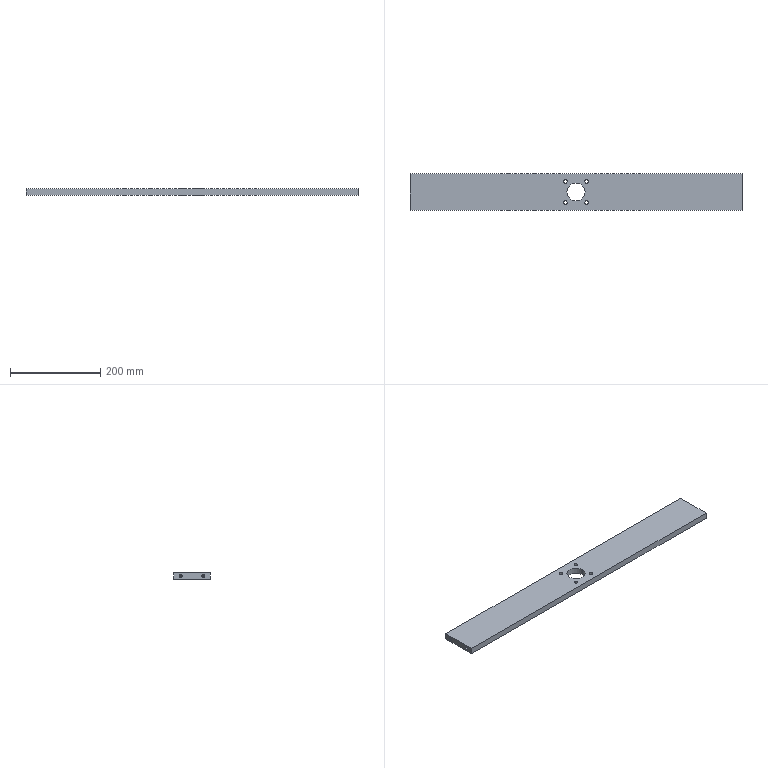Part | SolidWorks | features 3DProfileFeature 2, HoleWzd 2, Extrusion 1, ICE 1 | 1 solid | 32 faces | box 735 x 80 x 14 mm | volume 799824 mm3 | cylinder 18 | cone 8 | plane 6 | commonest cylinder face diameters 6.8 x8 8 x8 40 x2
STEP:
#1=CARTESIAN_POINT('',(715.25,15.,10.4));
#2=VERTEX_POINT('',#1);
#3=CARTESIAN_POINT('',(715.25,15.,3.6));
#4=VERTEX_POINT('',#3);
#5=CARTESIAN_POINT('',(715.25,15.,7.));
#6=DIRECTION('',(1.,0.,0.));
#7=DIRECTION('',(0.,0.,-1.));
#8=AXIS2_PLACEMENT_3D('',#5,#6,#7);
#9=CIRCLE('',#8,3.4);
#10=EDGE_CURVE('',#2,#4,#9,.T.);
#11=ORIENTED_EDGE('',*,*,#10,.F.);
#12=CARTESIAN_POINT('',(735.,15.,10.4));
#13=VERTEX_POINT('',#12);
#14=CARTESIAN_POINT('',(735.,15.,10.4));
#15=DIRECTION('',(1.,0.,0.));
#16=VECTOR('',#15,1000.);
#17=LINE('',#14,#16);
#18=EDGE_CURVE('',#2,#13,#17,.T.);
#19=ORIENTED_EDGE('',*,*,#18,.T.);
#20=CARTESIAN_POINT('',(735.,15.,3.6));
#21=VERTEX_POINT('',#20);
#22=CARTESIAN_POINT('',(735.,15.,7.));
#23=DIRECTION('',(1.,0.,0.));
#24=DIRECTION('',(0.,0.,-1.));
#25=AXIS2_PLACEMENT_3D('',#22,#23,#24);
#26=CIRCLE('',#25,3.4);
#27=EDGE_CURVE('',#13,#21,#26,.T.);
#28=ORIENTED_EDGE('',*,*,#27,.T.);
#29=CARTESIAN_POINT('',(735.,15.,3.6));
#30=DIRECTION('',(1.,0.,0.));
#31=VECTOR('',#30,1000.);
#32=LINE('',#29,#31);
#33=EDGE_CURVE('',#4,#21,#32,.T.);
#34=ORIENTED_EDGE('',*,*,#33,.F.);
#35=EDGE_LOOP('',(#11,#19,#28,#34));
#36=FACE_OUTER_BOUND('',#35,.T.);
#37=CARTESIAN_POINT('',(735.,15.,7.));
#38=DIRECTION('',(1.,0.,0.));
#39=DIRECTION('',(0.,0.,-1.));
#40=AXIS2_PLACEMENT_3D('',#37,#38,#39);
#41=CYLINDRICAL_SURFACE('',#40,3.4);
#42=ADVANCED_FACE('',(#36),#41,.F.);
#43=CARTESIAN_POINT('',(713.207,15.,7.));
#44=VERTEX_POINT('',#43);
#45=CARTESIAN_POINT('',(715.25,15.,3.6));
#46=DIRECTION('',(0.515,0.,-0.8572));
#47=VECTOR('',#46,1000.);
#48=LINE('',#45,#47);
#49=EDGE_CURVE('',#44,#4,#48,.T.);
#50=ORIENTED_EDGE('',*,*,#49,.F.);
#51=CARTESIAN_POINT('',(715.25,15.,10.4));
#52=DIRECTION('',(0.515,0.,0.8572));
#53=VECTOR('',#52,1000.);
#54=LINE('',#51,#53);
#55=EDGE_CURVE('',#44,#2,#54,.T.);
#56=ORIENTED_EDGE('',*,*,#55,.T.);
#57=ORIENTED_EDGE('',*,*,#10,.T.);
#58=EDGE_LOOP('',(#50,#56,#57));
#59=FACE_OUTER_BOUND('',#58,.T.);
#60=CARTESIAN_POINT('',(715.25,15.,7.));
#61=DIRECTION('',(1.,0.,0.));
#62=DIRECTION('',(0.,0.,-1.));
#63=AXIS2_PLACEMENT_3D('',#60,#61,#62);
#64=CONICAL_SURFACE('',#63,3.4,1.03);
#65=ADVANCED_FACE('',(#59),#64,.F.);
#66=CARTESIAN_POINT('',(715.25,65.,10.4));
#67=VERTEX_POINT('',#66);
#68=CARTESIAN_POINT('',(715.25,65.,3.6));
#69=VERTEX_POINT('',#68);
#70=CARTESIAN_POINT('',(715.25,65.,7.));
#71=DIRECTION('',(1.,0.,0.));
#72=DIRECTION('',(0.,0.,-1.));
#73=AXIS2_PLACEMENT_3D('',#70,#71,#72);
#74=CIRCLE('',#73,3.4);
#75=EDGE_CURVE('',#67,#69,#74,.T.);
#76=ORIENTED_EDGE('',*,*,#75,.F.);
#77=CARTESIAN_POINT('',(735.,65.,10.4));
#78=VERTEX_POINT('',#77);
#79=CARTESIAN_POINT('',(735.,65.,10.4));
#80=DIRECTION('',(1.,0.,0.));
#81=VECTOR('',#80,1000.);
#82=LINE('',#79,#81);
#83=EDGE_CURVE('',#67,#78,#82,.T.);
#84=ORIENTED_EDGE('',*,*,#83,.T.);
#85=CARTESIAN_POINT('',(735.,65.,3.6));
#86=VERTEX_POINT('',#85);
#87=CARTESIAN_POINT('',(735.,65.,7.));
#88=DIRECTION('',(1.,0.,0.));
#89=DIRECTION('',(0.,0.,-1.));
#90=AXIS2_PLACEMENT_3D('',#87,#88,#89);
#91=CIRCLE('',#90,3.4);
#92=EDGE_CURVE('',#78,#86,#91,.T.);
#93=ORIENTED_EDGE('',*,*,#92,.T.);
#94=CARTESIAN_POINT('',(735.,65.,3.6));
#95=DIRECTION('',(1.,0.,0.));
#96=VECTOR('',#95,1000.);
#97=LINE('',#94,#96);
#98=EDGE_CURVE('',#69,#86,#97,.T.);
#99=ORIENTED_EDGE('',*,*,#98,.F.);
#100=EDGE_LOOP('',(#76,#84,#93,#99));
#101=FACE_OUTER_BOUND('',#100,.T.);
#102=CARTESIAN_POINT('',(735.,65.,7.));
#103=DIRECTION('',(1.,0.,0.));
#104=DIRECTION('',(0.,0.,-1.));
#105=AXIS2_PLACEMENT_3D('',#102,#103,#104);
#106=CYLINDRICAL_SURFACE('',#105,3.4);
#107=ADVANCED_FACE('',(#101),#106,.F.);
#108=CARTESIAN_POINT('',(713.207,65.,7.));
#109=VERTEX_POINT('',#108);
#110=CARTESIAN_POINT('',(715.25,65.,3.6));
#111=DIRECTION('',(0.515,0.,-0.8572));
#112=VECTOR('',#111,1000.);
#113=LINE('',#110,#112);
#114=EDGE_CURVE('',#109,#69,#113,.T.);
#115=ORIENTED_EDGE('',*,*,#114,.F.);
#116=CARTESIAN_POINT('',(715.25,65.,10.4));
#117=DIRECTION('',(0.515,0.,0.8572));
#118=VECTOR('',#117,1000.);
#119=LINE('',#116,#118);
#120=EDGE_CURVE('',#109,#67,#119,.T.);
#121=ORIENTED_EDGE('',*,*,#120,.T.);
#122=ORIENTED_EDGE('',*,*,#75,.T.);
#123=EDGE_LOOP('',(#115,#121,#122));
#124=FACE_OUTER_BOUND('',#123,.T.);
#125=CARTESIAN_POINT('',(715.25,65.,7.));
#126=DIRECTION('',(1.,0.,0.));
#127=DIRECTION('',(0.,0.,-1.));
#128=AXIS2_PLACEMENT_3D('',#125,#126,#127);
#129=CONICAL_SURFACE('',#128,3.4,1.03);
#130=ADVANCED_FACE('',(#124),#129,.F.);
#131=CARTESIAN_POINT('',(19.75,65.,3.6));
#132=VERTEX_POINT('',#131);
#133=CARTESIAN_POINT('',(19.75,65.,10.4));
#134=VERTEX_POINT('',#133);
#135=CARTESIAN_POINT('',(19.75,65.,7.));
#136=DIRECTION('',(-1.,0.,0.));
#137=DIRECTION('',(0.,0.,1.));
#138=AXIS2_PLACEMENT_3D('',#135,#136,#137);
#139=CIRCLE('',#138,3.4);
#140=EDGE_CURVE('',#132,#134,#139,.T.);
#141=ORIENTED_EDGE('',*,*,#140,.F.);
#142=CARTESIAN_POINT('',(0.,65.,3.6));
#143=VERTEX_POINT('',#142);
#144=CARTESIAN_POINT('',(0.,65.,3.6));
#145=DIRECTION('',(-1.,0.,0.));
#146=VECTOR('',#145,1000.);
#147=LINE('',#144,#146);
#148=EDGE_CURVE('',#132,#143,#147,.T.);
#149=ORIENTED_EDGE('',*,*,#148,.T.);
#150=CARTESIAN_POINT('',(0.,65.,10.4));
#151=VERTEX_POINT('',#150);
#152=CARTESIAN_POINT('',(0.,65.,7.));
#153=DIRECTION('',(-1.,0.,0.));
#154=DIRECTION('',(0.,0.,1.));
#155=AXIS2_PLACEMENT_3D('',#152,#153,#154);
#156=CIRCLE('',#155,3.4);
#157=EDGE_CURVE('',#143,#151,#156,.T.);
#158=ORIENTED_EDGE('',*,*,#157,.T.);
#159=CARTESIAN_POINT('',(0.,65.,10.4));
#160=DIRECTION('',(-1.,0.,0.));
#161=VECTOR('',#160,1000.);
#162=LINE('',#159,#161);
#163=EDGE_CURVE('',#134,#151,#162,.T.);
#164=ORIENTED_EDGE('',*,*,#163,.F.);
#165=EDGE_LOOP('',(#141,#149,#158,#164));
#166=FACE_OUTER_BOUND('',#165,.T.);
#167=CARTESIAN_POINT('',(0.,65.,7.));
#168=DIRECTION('',(-1.,0.,0.));
#169=DIRECTION('',(0.,0.,1.));
#170=AXIS2_PLACEMENT_3D('',#167,#168,#169);
#171=CYLINDRICAL_SURFACE('',#170,3.4);
#172=ADVANCED_FACE('',(#166),#171,.F.);
#173=CARTESIAN_POINT('',(21.793,65.,7.));
#174=VERTEX_POINT('',#173);
#175=CARTESIAN_POINT('',(19.75,65.,10.4));
#176=DIRECTION('',(-0.515,0.,0.8572));
#177=VECTOR('',#176,1000.);
#178=LINE('',#175,#177);
#179=EDGE_CURVE('',#174,#134,#178,.T.);
#180=ORIENTED_EDGE('',*,*,#179,.F.);
#181=CARTESIAN_POINT('',(19.75,65.,3.6));
#182=DIRECTION('',(-0.515,0.,-0.8572));
#183=VECTOR('',#182,1000.);
#184=LINE('',#181,#183);
#185=EDGE_CURVE('',#174,#132,#184,.T.);
#186=ORIENTED_EDGE('',*,*,#185,.T.);
#187=ORIENTED_EDGE('',*,*,#140,.T.);
#188=EDGE_LOOP('',(#180,#186,#187));
#189=FACE_OUTER_BOUND('',#188,.T.);
#190=CARTESIAN_POINT('',(19.75,65.,7.));
#191=DIRECTION('',(-1.,0.,0.));
#192=DIRECTION('',(0.,0.,1.));
#193=AXIS2_PLACEMENT_3D('',#190,#191,#192);
#194=CONICAL_SURFACE('',#193,3.4,1.03);
#195=ADVANCED_FACE('',(#189),#194,.F.);
#196=CARTESIAN_POINT('',(19.75,15.,3.6));
#197=VERTEX_POINT('',#196);
#198=CARTESIAN_POINT('',(19.75,15.,10.4));
#199=VERTEX_POINT('',#198);
#200=CARTESIAN_POINT('',(19.75,15.,7.));
#201=DIRECTION('',(-1.,0.,0.));
#202=DIRECTION('',(0.,0.,1.));
#203=AXIS2_PLACEMENT_3D('',#200,#201,#202);
#204=CIRCLE('',#203,3.4);
#205=EDGE_CURVE('',#197,#199,#204,.T.);
#206=ORIENTED_EDGE('',*,*,#205,.F.);
#207=CARTESIAN_POINT('',(0.,15.,3.6));
#208=VERTEX_POINT('',#207);
#209=CARTESIAN_POINT('',(0.,15.,3.6));
#210=DIRECTION('',(-1.,0.,0.));
#211=VECTOR('',#210,1000.);
#212=LINE('',#209,#211);
#213=EDGE_CURVE('',#197,#208,#212,.T.);
#214=ORIENTED_EDGE('',*,*,#213,.T.);
#215=CARTESIAN_POINT('',(0.,15.,10.4));
#216=VERTEX_POINT('',#215);
#217=CARTESIAN_POINT('',(0.,15.,7.));
#218=DIRECTION('',(-1.,0.,0.));
#219=DIRECTION('',(0.,0.,1.));
#220=AXIS2_PLACEMENT_3D('',#217,#218,#219);
#221=CIRCLE('',#220,3.4);
#222=EDGE_CURVE('',#208,#216,#221,.T.);
#223=ORIENTED_EDGE('',*,*,#222,.T.);
#224=CARTESIAN_POINT('',(0.,15.,10.4));
#225=DIRECTION('',(-1.,0.,0.));
#226=VECTOR('',#225,1000.);
#227=LINE('',#224,#226);
#228=EDGE_CURVE('',#199,#216,#227,.T.);
#229=ORIENTED_EDGE('',*,*,#228,.F.);
#230=EDGE_LOOP('',(#206,#214,#223,#229));
#231=FACE_OUTER_BOUND('',#230,.T.);
#232=CARTESIAN_POINT('',(0.,15.,7.));
#233=DIRECTION('',(-1.,0.,0.));
#234=DIRECTION('',(0.,0.,1.));
#235=AXIS2_PLACEMENT_3D('',#232,#233,#234);
#236=CYLINDRICAL_SURFACE('',#235,3.4);
#237=ADVANCED_FACE('',(#231),#236,.F.);
#238=CARTESIAN_POINT('',(21.793,15.,7.));
#239=VERTEX_POINT('',#238);
#240=CARTESIAN_POINT('',(19.75,15.,10.4));
#241=DIRECTION('',(-0.515,0.,0.8572));
#242=VECTOR('',#241,1000.);
#243=LINE('',#240,#242);
#244=EDGE_CURVE('',#239,#199,#243,.T.);
#245=ORIENTED_EDGE('',*,*,#244,.F.);
#246=CARTESIAN_POINT('',(19.75,15.,3.6));
#247=DIRECTION('',(-0.515,0.,-0.8572));
#248=VECTOR('',#247,1000.);
#249=LINE('',#246,#248);
#250=EDGE_CURVE('',#239,#197,#249,.T.);
#251=ORIENTED_EDGE('',*,*,#250,.T.);
#252=ORIENTED_EDGE('',*,*,#205,.T.);
#253=EDGE_LOOP('',(#245,#251,#252));
#254=FACE_OUTER_BOUND('',#253,.T.);
#255=CARTESIAN_POINT('',(19.75,15.,7.));
#256=DIRECTION('',(-1.,0.,0.));
#257=DIRECTION('',(0.,0.,1.));
#258=AXIS2_PLACEMENT_3D('',#255,#256,#257);
#259=CONICAL_SURFACE('',#258,3.4,1.03);
#260=ADVANCED_FACE('',(#254),#259,.F.);
#261=CARTESIAN_POINT('',(340.,16.5,0.));
#262=VERTEX_POINT('',#261);
#263=CARTESIAN_POINT('',(348.,16.5,0.));
#264=VERTEX_POINT('',#263);
#265=CARTESIAN_POINT('',(344.,16.5,0.));
#266=DIRECTION('',(0.,0.,1.));
#267=DIRECTION('',(1.,0.,0.));
#268=AXIS2_PLACEMENT_3D('',#265,#266,#267);
#269=CIRCLE('',#268,4.);
#270=EDGE_CURVE('',#262,#264,#269,.T.);
#271=ORIENTED_EDGE('',*,*,#270,.F.);
#272=CARTESIAN_POINT('',(340.,16.5,14.));
#273=VERTEX_POINT('',#272);
#274=CARTESIAN_POINT('',(340.,16.5,0.));
#275=DIRECTION('',(0.,0.,1.));
#276=VECTOR('',#275,1000.);
#277=LINE('',#274,#276);
#278=EDGE_CURVE('',#262,#273,#277,.T.);
#279=ORIENTED_EDGE('',*,*,#278,.T.);
#280=CARTESIAN_POINT('',(348.,16.5,14.));
#281=VERTEX_POINT('',#280);
#282=CARTESIAN_POINT('',(344.,16.5,14.));
#283=DIRECTION('',(0.,0.,1.));
#284=DIRECTION('',(1.,0.,0.));
#285=AXIS2_PLACEMENT_3D('',#282,#283,#284);
#286=CIRCLE('',#285,4.);
#287=EDGE_CURVE('',#273,#281,#286,.T.);
#288=ORIENTED_EDGE('',*,*,#287,.T.);
#289=CARTESIAN_POINT('',(348.,16.5,0.));
#290=DIRECTION('',(0.,0.,1.));
#291=VECTOR('',#290,1000.);
#292=LINE('',#289,#291);
#293=EDGE_CURVE('',#264,#281,#292,.T.);
#294=ORIENTED_EDGE('',*,*,#293,.F.);
#295=EDGE_LOOP('',(#271,#279,#288,#294));
#296=FACE_OUTER_BOUND('',#295,.T.);
#297=CARTESIAN_POINT('',(344.,16.5,0.));
#298=DIRECTION('',(0.,0.,1.));
#299=DIRECTION('',(1.,0.,0.));
#300=AXIS2_PLACEMENT_3D('',#297,#298,#299);
#301=CYLINDRICAL_SURFACE('',#300,4.);
#302=ADVANCED_FACE('',(#296),#301,.F.);
#303=CARTESIAN_POINT('',(387.,16.5,0.));
#304=VERTEX_POINT('',#303);
#305=CARTESIAN_POINT('',(395.,16.5,0.));
#306=VERTEX_POINT('',#305);
#307=CARTESIAN_POINT('',(391.,16.5,0.));
#308=DIRECTION('',(0.,0.,1.));
#309=DIRECTION('',(1.,0.,0.));
#310=AXIS2_PLACEMENT_3D('',#307,#308,#309);
#311=CIRCLE('',#310,4.);
#312=EDGE_CURVE('',#304,#306,#311,.T.);
#313=ORIENTED_EDGE('',*,*,#312,.F.);
#314=CARTESIAN_POINT('',(387.,16.5,14.));
#315=VERTEX_POINT('',#314);
#316=CARTESIAN_POINT('',(387.,16.5,0.));
#317=DIRECTION('',(0.,0.,1.));
#318=VECTOR('',#317,1000.);
#319=LINE('',#316,#318);
#320=EDGE_CURVE('',#304,#315,#319,.T.);
#321=ORIENTED_EDGE('',*,*,#320,.T.);
#322=CARTESIAN_POINT('',(395.,16.5,14.));
#323=VERTEX_POINT('',#322);
#324=CARTESIAN_POINT('',(391.,16.5,14.));
#325=DIRECTION('',(0.,0.,1.));
#326=DIRECTION('',(1.,0.,0.));
#327=AXIS2_PLACEMENT_3D('',#324,#325,#326);
#328=CIRCLE('',#327,4.);
#329=EDGE_CURVE('',#315,#323,#328,.T.);
#330=ORIENTED_EDGE('',*,*,#329,.T.);
#331=CARTESIAN_POINT('',(395.,16.5,0.));
#332=DIRECTION('',(0.,0.,1.));
#333=VECTOR('',#332,1000.);
#334=LINE('',#331,#333);
#335=EDGE_CURVE('',#306,#323,#334,.T.);
#336=ORIENTED_EDGE('',*,*,#335,.F.);
#337=EDGE_LOOP('',(#313,#321,#330,#336));
#338=FACE_OUTER_BOUND('',#337,.T.);
#339=CARTESIAN_POINT('',(391.,16.5,0.));
#340=DIRECTION('',(0.,0.,1.));
#341=DIRECTION('',(1.,0.,0.));
#342=AXIS2_PLACEMENT_3D('',#339,#340,#341);
#343=CYLINDRICAL_SURFACE('',#342,4.);
#344=ADVANCED_FACE('',(#338),#343,.F.);
#345=CARTESIAN_POINT('',(347.5,40.,0.));
#346=VERTEX_POINT('',#345);
#347=CARTESIAN_POINT('',(387.5,40.,0.));
#348=VERTEX_POINT('',#347);
#349=CARTESIAN_POINT('',(367.5,40.,0.));
#350=DIRECTION('',(0.,0.,1.));
#351=DIRECTION('',(1.,0.,0.));
#352=AXIS2_PLACEMENT_3D('',#349,#350,#351);
#353=CIRCLE('',#352,20.);
#354=EDGE_CURVE('',#346,#348,#353,.T.);
#355=ORIENTED_EDGE('',*,*,#354,.F.);
#356=CARTESIAN_POINT('',(347.5,40.,14.));
#357=VERTEX_POINT('',#356);
#358=CARTESIAN_POINT('',(347.5,40.,0.));
#359=DIRECTION('',(0.,0.,1.));
#360=VECTOR('',#359,1000.);
#361=LINE('',#358,#360);
#362=EDGE_CURVE('',#346,#357,#361,.T.);
#363=ORIENTED_EDGE('',*,*,#362,.T.);
#364=CARTESIAN_POINT('',(387.5,40.,14.));
#365=VERTEX_POINT('',#364);
#366=CARTESIAN_POINT('',(367.5,40.,14.));
#367=DIRECTION('',(0.,0.,1.));
#368=DIRECTION('',(1.,0.,0.));
#369=AXIS2_PLACEMENT_3D('',#366,#367,#368);
#370=CIRCLE('',#369,20.);
#371=EDGE_CURVE('',#357,#365,#370,.T.);
#372=ORIENTED_EDGE('',*,*,#371,.T.);
#373=CARTESIAN_POINT('',(387.5,40.,0.));
#374=DIRECTION('',(0.,0.,1.));
#375=VECTOR('',#374,1000.);
#376=LINE('',#373,#375);
#377=EDGE_CURVE('',#348,#365,#376,.T.);
#378=ORIENTED_EDGE('',*,*,#377,.F.);
#379=EDGE_LOOP('',(#355,#363,#372,#378));
#380=FACE_OUTER_BOUND('',#379,.T.);
#381=CARTESIAN_POINT('',(367.5,40.,0.));
#382=DIRECTION('',(0.,0.,1.));
#383=DIRECTION('',(1.,0.,0.));
#384=AXIS2_PLACEMENT_3D('',#381,#382,#383);
#385=CYLINDRICAL_SURFACE('',#384,20.);
#386=ADVANCED_FACE('',(#380),#385,.F.);
#387=CARTESIAN_POINT('',(387.,63.5,0.));
#388=VERTEX_POINT('',#387);
#389=CARTESIAN_POINT('',(395.,63.5,0.));
#390=VERTEX_POINT('',#389);
#391=CARTESIAN_POINT('',(391.,63.5,0.));
#392=DIRECTION('',(0.,0.,1.));
#393=DIRECTION('',(1.,0.,0.));
#394=AXIS2_PLACEMENT_3D('',#391,#392,#393);
#395=CIRCLE('',#394,4.);
#396=EDGE_CURVE('',#388,#390,#395,.T.);
#397=ORIENTED_EDGE('',*,*,#396,.F.);
#398=CARTESIAN_POINT('',(387.,63.5,14.));
#399=VERTEX_POINT('',#398);
#400=CARTESIAN_POINT('',(387.,63.5,0.));
#401=DIRECTION('',(0.,0.,1.));
#402=VECTOR('',#401,1000.);
#403=LINE('',#400,#402);
#404=EDGE_CURVE('',#388,#399,#403,.T.);
#405=ORIENTED_EDGE('',*,*,#404,.T.);
#406=CARTESIAN_POINT('',(395.,63.5,14.));
#407=VERTEX_POINT('',#406);
#408=CARTESIAN_POINT('',(391.,63.5,14.));
#409=DIRECTION('',(0.,0.,1.));
#410=DIRECTION('',(1.,0.,0.));
#411=AXIS2_PLACEMENT_3D('',#408,#409,#410);
#412=CIRCLE('',#411,4.);
#413=EDGE_CURVE('',#399,#407,#412,.T.);
#414=ORIENTED_EDGE('',*,*,#413,.T.);
#415=CARTESIAN_POINT('',(395.,63.5,0.));
#416=DIRECTION('',(0.,0.,1.));
#417=VECTOR('',#416,1000.);
#418=LINE('',#415,#417);
#419=EDGE_CURVE('',#390,#407,#418,.T.);
#420=ORIENTED_EDGE('',*,*,#419,.F.);
#421=EDGE_LOOP('',(#397,#405,#414,#420));
#422=FACE_OUTER_BOUND('',#421,.T.);
#423=CARTESIAN_POINT('',(391.,63.5,0.));
#424=DIRECTION('',(0.,0.,1.));
#425=DIRECTION('',(1.,0.,0.));
#426=AXIS2_PLACEMENT_3D('',#423,#424,#425);
#427=CYLINDRICAL_SURFACE('',#426,4.);
#428=ADVANCED_FACE('',(#422),#427,.F.);
#429=CARTESIAN_POINT('',(340.,63.5,0.));
#430=VERTEX_POINT('',#429);
#431=CARTESIAN_POINT('',(348.,63.5,0.));
#432=VERTEX_POINT('',#431);
#433=CARTESIAN_POINT('',(344.,63.5,0.));
#434=DIRECTION('',(0.,0.,1.));
#435=DIRECTION('',(1.,0.,0.));
#436=AXIS2_PLACEMENT_3D('',#433,#434,#435);
#437=CIRCLE('',#436,4.);
#438=EDGE_CURVE('',#430,#432,#437,.T.);
#439=ORIENTED_EDGE('',*,*,#438,.F.);
#440=CARTESIAN_POINT('',(340.,63.5,14.));
#441=VERTEX_POINT('',#440);
#442=CARTESIAN_POINT('',(340.,63.5,0.));
#443=DIRECTION('',(0.,0.,1.));
#444=VECTOR('',#443,1000.);
#445=LINE('',#442,#444);
#446=EDGE_CURVE('',#430,#441,#445,.T.);
#447=ORIENTED_EDGE('',*,*,#446,.T.);
#448=CARTESIAN_POINT('',(348.,63.5,14.));
#449=VERTEX_POINT('',#448);
#450=CARTESIAN_POINT('',(344.,63.5,14.));
#451=DIRECTION('',(0.,0.,1.));
#452=DIRECTION('',(1.,0.,0.));
#453=AXIS2_PLACEMENT_3D('',#450,#451,#452);
#454=CIRCLE('',#453,4.);
#455=EDGE_CURVE('',#441,#449,#454,.T.);
#456=ORIENTED_EDGE('',*,*,#455,.T.);
#457=CARTESIAN_POINT('',(348.,63.5,0.));
#458=DIRECTION('',(0.,0.,1.));
#459=VECTOR('',#458,1000.);
#460=LINE('',#457,#459);
#461=EDGE_CURVE('',#432,#449,#460,.T.);
#462=ORIENTED_EDGE('',*,*,#461,.F.);
#463=EDGE_LOOP('',(#439,#447,#456,#462));
#464=FACE_OUTER_BOUND('',#463,.T.);
#465=CARTESIAN_POINT('',(344.,63.5,0.));
#466=DIRECTION('',(0.,0.,1.));
#467=DIRECTION('',(1.,0.,0.));
#468=AXIS2_PLACEMENT_3D('',#465,#466,#467);
#469=CYLINDRICAL_SURFACE('',#468,4.);
#470=ADVANCED_FACE('',(#464),#469,.F.);
#471=CARTESIAN_POINT('',(0.,65.,7.));
#472=DIRECTION('',(-1.,0.,0.));
#473=DIRECTION('',(0.,0.,1.));
#474=AXIS2_PLACEMENT_3D('',#471,#472,#473);
#475=CIRCLE('',#474,3.4);
#476=EDGE_CURVE('',#151,#143,#475,.T.);
#477=ORIENTED_EDGE('',*,*,#476,.F.);
#478=ORIENTED_EDGE('',*,*,#157,.F.);
#479=EDGE_LOOP('',(#477,#478));
#480=FACE_BOUND('',#479,.T.);
#481=CARTESIAN_POINT('',(0.,15.,7.));
#482=DIRECTION('',(-1.,0.,0.));
#483=DIRECTION('',(0.,0.,1.));
#484=AXIS2_PLACEMENT_3D('',#481,#482,#483);
#485=CIRCLE('',#484,3.4);
#486=EDGE_CURVE('',#216,#208,#485,.T.);
#487=ORIENTED_EDGE('',*,*,#486,.F.);
#488=ORIENTED_EDGE('',*,*,#222,.F.);
#489=EDGE_LOOP('',(#487,#488));
#490=FACE_BOUND('',#489,.T.);
#491=CARTESIAN_POINT('',(0.,80.,0.));
#492=VERTEX_POINT('',#491);
#493=CARTESIAN_POINT('',(0.,0.,0.));
#494=VERTEX_POINT('',#493);
#495=CARTESIAN_POINT('',(0.,0.,0.));
#496=DIRECTION('',(0.,-1.,0.));
#497=VECTOR('',#496,1000.);
#498=LINE('',#495,#497);
#499=EDGE_CURVE('',#492,#494,#498,.T.);
#500=ORIENTED_EDGE('',*,*,#499,.T.);
#501=CARTESIAN_POINT('',(0.,0.,14.));
#502=VERTEX_POINT('',#501);
#503=CARTESIAN_POINT('',(0.,0.,14.));
#504=DIRECTION('',(0.,0.,-1.));
#505=VECTOR('',#504,1000.);
#506=LINE('',#503,#505);
#507=EDGE_CURVE('',#502,#494,#506,.T.);
#508=ORIENTED_EDGE('',*,*,#507,.F.);
#509=CARTESIAN_POINT('',(0.,80.,14.));
#510=VERTEX_POINT('',#509);
#511=CARTESIAN_POINT('',(0.,0.,14.));
#512=DIRECTION('',(0.,-1.,0.));
#513=VECTOR('',#512,1000.);
#514=LINE('',#511,#513);
#515=EDGE_CURVE('',#510,#502,#514,.T.);
#516=ORIENTED_EDGE('',*,*,#515,.F.);
#517=CARTESIAN_POINT('',(0.,80.,14.));
#518=DIRECTION('',(0.,0.,-1.));
#519=VECTOR('',#518,1000.);
#520=LINE('',#517,#519);
#521=EDGE_CURVE('',#510,#492,#520,.T.);
#522=ORIENTED_EDGE('',*,*,#521,.T.);
#523=EDGE_LOOP('',(#500,#508,#516,#522));
#524=FACE_OUTER_BOUND('',#523,.T.);
#525=CARTESIAN_POINT('',(0.,0.,14.));
#526=DIRECTION('',(1.,0.,0.));
#527=DIRECTION('',(0.,0.,-1.));
#528=AXIS2_PLACEMENT_3D('',#525,#526,#527);
#529=PLANE('',#528);
#530=ADVANCED_FACE('',(#480,#490,#524),#529,.F.);
#531=CARTESIAN_POINT('',(735.,0.,0.));
#532=VERTEX_POINT('',#531);
#533=CARTESIAN_POINT('',(0.,0.,0.));
#534=DIRECTION('',(1.,0.,0.));
#535=VECTOR('',#534,1000.);
#536=LINE('',#533,#535);
#537=EDGE_CURVE('',#494,#532,#536,.T.);
#538=ORIENTED_EDGE('',*,*,#537,.T.);
#539=CARTESIAN_POINT('',(735.,0.,14.));
#540=VERTEX_POINT('',#539);
#541=CARTESIAN_POINT('',(735.,0.,14.));
#542=DIRECTION('',(0.,0.,-1.));
#543=VECTOR('',#542,1000.);
#544=LINE('',#541,#543);
#545=EDGE_CURVE('',#540,#532,#544,.T.);
#546=ORIENTED_EDGE('',*,*,#545,.F.);
#547=CARTESIAN_POINT('',(0.,0.,14.));
#548=DIRECTION('',(1.,0.,0.));
#549=VECTOR('',#548,1000.);
#550=LINE('',#547,#549);
#551=EDGE_CURVE('',#502,#540,#550,.T.);
#552=ORIENTED_EDGE('',*,*,#551,.F.);
#553=ORIENTED_EDGE('',*,*,#507,.T.);
#554=EDGE_LOOP('',(#538,#546,#552,#553));
#555=FACE_OUTER_BOUND('',#554,.T.);
#556=CARTESIAN_POINT('',(0.,0.,14.));
#557=DIRECTION('',(0.,1.,0.));
#558=DIRECTION('',(0.,0.,1.));
#559=AXIS2_PLACEMENT_3D('',#556,#557,#558);
#560=PLANE('',#559);
#561=ADVANCED_FACE('',(#555),#560,.F.);
#562=CARTESIAN_POINT('',(735.,15.,7.));
#563=DIRECTION('',(1.,0.,0.));
#564=DIRECTION('',(0.,0.,-1.));
#565=AXIS2_PLACEMENT_3D('',#562,#563,#564);
#566=CIRCLE('',#565,3.4);
#567=EDGE_CURVE('',#21,#13,#566,.T.);
#568=ORIENTED_EDGE('',*,*,#567,.F.);
#569=ORIENTED_EDGE('',*,*,#27,.F.);
#570=EDGE_LOOP('',(#568,#569));
#571=FACE_BOUND('',#570,.T.);
#572=CARTESIAN_POINT('',(735.,65.,7.));
#573=DIRECTION('',(1.,0.,0.));
#574=DIRECTION('',(0.,0.,-1.));
#575=AXIS2_PLACEMENT_3D('',#572,#573,#574);
#576=CIRCLE('',#575,3.4);
#577=EDGE_CURVE('',#86,#78,#576,.T.);
#578=ORIENTED_EDGE('',*,*,#577,.F.);
#579=ORIENTED_EDGE('',*,*,#92,.F.);
#580=EDGE_LOOP('',(#578,#579));
#581=FACE_BOUND('',#580,.T.);
#582=CARTESIAN_POINT('',(735.,80.,0.));
#583=VERTEX_POINT('',#582);
#584=CARTESIAN_POINT('',(735.,0.,0.));
#585=DIRECTION('',(0.,1.,0.));
#586=VECTOR('',#585,1000.);
#587=LINE('',#584,#586);
#588=EDGE_CURVE('',#532,#583,#587,.T.);
#589=ORIENTED_EDGE('',*,*,#588,.T.);
#590=CARTESIAN_POINT('',(735.,80.,14.));
#591=VERTEX_POINT('',#590);
#592=CARTESIAN_POINT('',(735.,80.,14.));
#593=DIRECTION('',(0.,0.,-1.));
#594=VECTOR('',#593,1000.);
#595=LINE('',#592,#594);
#596=EDGE_CURVE('',#591,#583,#595,.T.);
#597=ORIENTED_EDGE('',*,*,#596,.F.);
#598=CARTESIAN_POINT('',(735.,0.,14.));
#599=DIRECTION('',(0.,1.,0.));
#600=VECTOR('',#599,1000.);
#601=LINE('',#598,#600);
#602=EDGE_CURVE('',#540,#591,#601,.T.);
#603=ORIENTED_EDGE('',*,*,#602,.F.);
#604=ORIENTED_EDGE('',*,*,#545,.T.);
#605=EDGE_LOOP('',(#589,#597,#603,#604));
#606=FACE_OUTER_BOUND('',#605,.T.);
#607=CARTESIAN_POINT('',(735.,0.,14.));
#608=DIRECTION('',(-1.,0.,0.));
#609=DIRECTION('',(0.,0.,1.));
#610=AXIS2_PLACEMENT_3D('',#607,#608,#609);
#611=PLANE('',#610);
#612=ADVANCED_FACE('',(#571,#581,#606),#611,.F.);
#613=CARTESIAN_POINT('',(0.,80.,0.));
#614=DIRECTION('',(-1.,0.,0.));
#615=VECTOR('',#614,1000.);
#616=LINE('',#613,#615);
#617=EDGE_CURVE('',#583,#492,#616,.T.);
#618=ORIENTED_EDGE('',*,*,#617,.T.);
#619=ORIENTED_EDGE('',*,*,#521,.F.);
#620=CARTESIAN_POINT('',(0.,80.,14.));
#621=DIRECTION('',(-1.,0.,0.));
#622=VECTOR('',#621,1000.);
#623=LINE('',#620,#622);
#624=EDGE_CURVE('',#591,#510,#623,.T.);
#625=ORIENTED_EDGE('',*,*,#624,.F.);
#626=ORIENTED_EDGE('',*,*,#596,.T.);
#627=EDGE_LOOP('',(#618,#619,#625,#626));
#628=FACE_OUTER_BOUND('',#627,.T.);
#629=CARTESIAN_POINT('',(0.,80.,14.));
#630=DIRECTION('',(0.,-1.,0.));
#631=DIRECTION('',(0.,0.,-1.));
#632=AXIS2_PLACEMENT_3D('',#629,#630,#631);
#633=PLANE('',#632);
#634=ADVANCED_FACE('',(#628),#633,.F.);
#635=CARTESIAN_POINT('',(344.,16.5,14.));
#636=DIRECTION('',(0.,0.,1.));
#637=DIRECTION('',(1.,0.,0.));
#638=AXIS2_PLACEMENT_3D('',#635,#636,#637);
#639=CIRCLE('',#638,4.);
#640=EDGE_CURVE('',#281,#273,#639,.T.);
#641=ORIENTED_EDGE('',*,*,#640,.F.);
#642=ORIENTED_EDGE('',*,*,#287,.F.);
#643=EDGE_LOOP('',(#641,#642));
#644=FACE_BOUND('',#643,.T.);
#645=CARTESIAN_POINT('',(391.,16.5,14.));
#646=DIRECTION('',(0.,0.,1.));
#647=DIRECTION('',(1.,0.,0.));
#648=AXIS2_PLACEMENT_3D('',#645,#646,#647);
#649=CIRCLE('',#648,4.);
#650=EDGE_CURVE('',#323,#315,#649,.T.);
#651=ORIENTED_EDGE('',*,*,#650,.F.);
#652=ORIENTED_EDGE('',*,*,#329,.F.);
#653=EDGE_LOOP('',(#651,#652));
#654=FACE_BOUND('',#653,.T.);
#655=CARTESIAN_POINT('',(367.5,40.,14.));
#656=DIRECTION('',(0.,0.,1.));
#657=DIRECTION('',(1.,0.,0.));
#658=AXIS2_PLACEMENT_3D('',#655,#656,#657);
#659=CIRCLE('',#658,20.);
#660=EDGE_CURVE('',#365,#357,#659,.T.);
#661=ORIENTED_EDGE('',*,*,#660,.F.);
#662=ORIENTED_EDGE('',*,*,#371,.F.);
#663=EDGE_LOOP('',(#661,#662));
#664=FACE_BOUND('',#663,.T.);
#665=CARTESIAN_POINT('',(391.,63.5,14.));
#666=DIRECTION('',(0.,0.,1.));
#667=DIRECTION('',(1.,0.,0.));
#668=AXIS2_PLACEMENT_3D('',#665,#666,#667);
#669=CIRCLE('',#668,4.);
#670=EDGE_CURVE('',#407,#399,#669,.T.);
#671=ORIENTED_EDGE('',*,*,#670,.F.);
#672=ORIENTED_EDGE('',*,*,#413,.F.);
#673=EDGE_LOOP('',(#671,#672));
#674=FACE_BOUND('',#673,.T.);
#675=CARTESIAN_POINT('',(344.,63.5,14.));
#676=DIRECTION('',(0.,0.,1.));
#677=DIRECTION('',(1.,0.,0.));
#678=AXIS2_PLACEMENT_3D('',#675,#676,#677);
#679=CIRCLE('',#678,4.);
#680=EDGE_CURVE('',#449,#441,#679,.T.);
#681=ORIENTED_EDGE('',*,*,#680,.F.);
#682=ORIENTED_EDGE('',*,*,#455,.F.);
#683=EDGE_LOOP('',(#681,#682));
#684=FACE_BOUND('',#683,.T.);
#685=ORIENTED_EDGE('',*,*,#515,.T.);
#686=ORIENTED_EDGE('',*,*,#551,.T.);
#687=ORIENTED_EDGE('',*,*,#602,.T.);
#688=ORIENTED_EDGE('',*,*,#624,.T.);
#689=EDGE_LOOP('',(#685,#686,#687,#688));
#690=FACE_OUTER_BOUND('',#689,.T.);
#691=CARTESIAN_POINT('',(0.,0.,14.));
#692=DIRECTION('',(0.,0.,-1.));
#693=DIRECTION('',(-1.,0.,0.));
#694=AXIS2_PLACEMENT_3D('',#691,#692,#693);
#695=PLANE('',#694);
#696=ADVANCED_FACE('',(#644,#654,#664,#674,#684,#690),#695,.F.);
#697=CARTESIAN_POINT('',(344.,16.5,0.));
#698=DIRECTION('',(0.,0.,1.));
#699=DIRECTION('',(1.,0.,0.));
#700=AXIS2_PLACEMENT_3D('',#697,#698,#699);
#701=CIRCLE('',#700,4.);
#702=EDGE_CURVE('',#264,#262,#701,.T.);
#703=ORIENTED_EDGE('',*,*,#702,.T.);
#704=ORIENTED_EDGE('',*,*,#270,.T.);
#705=EDGE_LOOP('',(#703,#704));
#706=FACE_BOUND('',#705,.T.);
#707=CARTESIAN_POINT('',(391.,16.5,0.));
#708=DIRECTION('',(0.,0.,1.));
#709=DIRECTION('',(1.,0.,0.));
#710=AXIS2_PLACEMENT_3D('',#707,#708,#709);
#711=CIRCLE('',#710,4.);
#712=EDGE_CURVE('',#306,#304,#711,.T.);
#713=ORIENTED_EDGE('',*,*,#712,.T.);
#714=ORIENTED_EDGE('',*,*,#312,.T.);
#715=EDGE_LOOP('',(#713,#714));
#716=FACE_BOUND('',#715,.T.);
#717=CARTESIAN_POINT('',(367.5,40.,0.));
#718=DIRECTION('',(0.,0.,1.));
#719=DIRECTION('',(1.,0.,0.));
#720=AXIS2_PLACEMENT_3D('',#717,#718,#719);
#721=CIRCLE('',#720,20.);
#722=EDGE_CURVE('',#348,#346,#721,.T.);
#723=ORIENTED_EDGE('',*,*,#722,.T.);
#724=ORIENTED_EDGE('',*,*,#354,.T.);
#725=EDGE_LOOP('',(#723,#724));
#726=FACE_BOUND('',#725,.T.);
#727=CARTESIAN_POINT('',(391.,63.5,0.));
#728=DIRECTION('',(0.,0.,1.));
#729=DIRECTION('',(1.,0.,0.));
#730=AXIS2_PLACEMENT_3D('',#727,#728,#729);
#731=CIRCLE('',#730,4.);
#732=EDGE_CURVE('',#390,#388,#731,.T.);
#733=ORIENTED_EDGE('',*,*,#732,.T.);
#734=ORIENTED_EDGE('',*,*,#396,.T.);
#735=EDGE_LOOP('',(#733,#734));
#736=FACE_BOUND('',#735,.T.);
#737=CARTESIAN_POINT('',(344.,63.5,0.));
#738=DIRECTION('',(0.,0.,1.));
#739=DIRECTION('',(1.,0.,0.));
#740=AXIS2_PLACEMENT_3D('',#737,#738,#739);
#741=CIRCLE('',#740,4.);
#742=EDGE_CURVE('',#432,#430,#741,.T.);
#743=ORIENTED_EDGE('',*,*,#742,.T.);
#744=ORIENTED_EDGE('',*,*,#438,.T.);
#745=EDGE_LOOP('',(#743,#744));
#746=FACE_BOUND('',#745,.T.);
#747=ORIENTED_EDGE('',*,*,#499,.F.);
#748=ORIENTED_EDGE('',*,*,#617,.F.);
#749=ORIENTED_EDGE('',*,*,#588,.F.);
#750=ORIENTED_EDGE('',*,*,#537,.F.);
#751=EDGE_LOOP('',(#747,#748,#749,#750));
#752=FACE_OUTER_BOUND('',#751,.T.);
#753=CARTESIAN_POINT('',(0.,0.,0.));
#754=DIRECTION('',(0.,0.,-1.));
#755=DIRECTION('',(-1.,0.,0.));
#756=AXIS2_PLACEMENT_3D('',#753,#754,#755);
#757=PLANE('',#756);
#758=ADVANCED_FACE('',(#706,#716,#726,#736,#746,#752),#757,.T.);
#759=ORIENTED_EDGE('',*,*,#446,.F.);
#760=ORIENTED_EDGE('',*,*,#742,.F.);
#761=ORIENTED_EDGE('',*,*,#461,.T.);
#762=ORIENTED_EDGE('',*,*,#680,.T.);
#763=EDGE_LOOP('',(#759,#760,#761,#762));
#764=FACE_OUTER_BOUND('',#763,.T.);
#765=CARTESIAN_POINT('',(344.,63.5,0.));
#766=DIRECTION('',(0.,0.,1.));
#767=DIRECTION('',(1.,0.,0.));
#768=AXIS2_PLACEMENT_3D('',#765,#766,#767);
#769=CYLINDRICAL_SURFACE('',#768,4.);
#770=ADVANCED_FACE('',(#764),#769,.F.);
#771=ORIENTED_EDGE('',*,*,#404,.F.);
#772=ORIENTED_EDGE('',*,*,#732,.F.);
#773=ORIENTED_EDGE('',*,*,#419,.T.);
#774=ORIENTED_EDGE('',*,*,#670,.T.);
#775=EDGE_LOOP('',(#771,#772,#773,#774));
#776=FACE_OUTER_BOUND('',#775,.T.);
#777=CARTESIAN_POINT('',(391.,63.5,0.));
#778=DIRECTION('',(0.,0.,1.));
#779=DIRECTION('',(1.,0.,0.));
#780=AXIS2_PLACEMENT_3D('',#777,#778,#779);
#781=CYLINDRICAL_SURFACE('',#780,4.);
#782=ADVANCED_FACE('',(#776),#781,.F.);
#783=ORIENTED_EDGE('',*,*,#362,.F.);
#784=ORIENTED_EDGE('',*,*,#722,.F.);
#785=ORIENTED_EDGE('',*,*,#377,.T.);
#786=ORIENTED_EDGE('',*,*,#660,.T.);
#787=EDGE_LOOP('',(#783,#784,#785,#786));
#788=FACE_OUTER_BOUND('',#787,.T.);
#789=CARTESIAN_POINT('',(367.5,40.,0.));
#790=DIRECTION('',(0.,0.,1.));
#791=DIRECTION('',(1.,0.,0.));
#792=AXIS2_PLACEMENT_3D('',#789,#790,#791);
#793=CYLINDRICAL_SURFACE('',#792,20.);
#794=ADVANCED_FACE('',(#788),#793,.F.);
#795=ORIENTED_EDGE('',*,*,#320,.F.);
#796=ORIENTED_EDGE('',*,*,#712,.F.);
#797=ORIENTED_EDGE('',*,*,#335,.T.);
#798=ORIENTED_EDGE('',*,*,#650,.T.);
#799=EDGE_LOOP('',(#795,#796,#797,#798));
#800=FACE_OUTER_BOUND('',#799,.T.);
#801=CARTESIAN_POINT('',(391.,16.5,0.));
#802=DIRECTION('',(0.,0.,1.));
#803=DIRECTION('',(1.,0.,0.));
#804=AXIS2_PLACEMENT_3D('',#801,#802,#803);
#805=CYLINDRICAL_SURFACE('',#804,4.);
#806=ADVANCED_FACE('',(#800),#805,.F.);
#807=ORIENTED_EDGE('',*,*,#278,.F.);
#808=ORIENTED_EDGE('',*,*,#702,.F.);
#809=ORIENTED_EDGE('',*,*,#293,.T.);
#810=ORIENTED_EDGE('',*,*,#640,.T.);
#811=EDGE_LOOP('',(#807,#808,#809,#810));
#812=FACE_OUTER_BOUND('',#811,.T.);
#813=CARTESIAN_POINT('',(344.,16.5,0.));
#814=DIRECTION('',(0.,0.,1.));
#815=DIRECTION('',(1.,0.,0.));
#816=AXIS2_PLACEMENT_3D('',#813,#814,#815);
#817=CYLINDRICAL_SURFACE('',#816,4.);
#818=ADVANCED_FACE('',(#812),#817,.F.);
#819=ORIENTED_EDGE('',*,*,#250,.F.);
#820=ORIENTED_EDGE('',*,*,#244,.T.);
#821=CARTESIAN_POINT('',(19.75,15.,7.));
#822=DIRECTION('',(-1.,0.,0.));
#823=DIRECTION('',(0.,0.,1.));
#824=AXIS2_PLACEMENT_3D('',#821,#822,#823);
#825=CIRCLE('',#824,3.4);
#826=EDGE_CURVE('',#199,#197,#825,.T.);
#827=ORIENTED_EDGE('',*,*,#826,.T.);
#828=EDGE_LOOP('',(#819,#820,#827));
#829=FACE_OUTER_BOUND('',#828,.T.);
#830=CARTESIAN_POINT('',(19.75,15.,7.));
#831=DIRECTION('',(-1.,0.,0.));
#832=DIRECTION('',(0.,0.,1.));
#833=AXIS2_PLACEMENT_3D('',#830,#831,#832);
#834=CONICAL_SURFACE('',#833,3.4,1.03);
#835=ADVANCED_FACE('',(#829),#834,.F.);
#836=ORIENTED_EDGE('',*,*,#213,.F.);
#837=ORIENTED_EDGE('',*,*,#826,.F.);
#838=ORIENTED_EDGE('',*,*,#228,.T.);
#839=ORIENTED_EDGE('',*,*,#486,.T.);
#840=EDGE_LOOP('',(#836,#837,#838,#839));
#841=FACE_OUTER_BOUND('',#840,.T.);
#842=CARTESIAN_POINT('',(0.,15.,7.));
#843=DIRECTION('',(-1.,0.,0.));
#844=DIRECTION('',(0.,0.,1.));
#845=AXIS2_PLACEMENT_3D('',#842,#843,#844);
#846=CYLINDRICAL_SURFACE('',#845,3.4);
#847=ADVANCED_FACE('',(#841),#846,.F.);
#848=ORIENTED_EDGE('',*,*,#185,.F.);
#849=ORIENTED_EDGE('',*,*,#179,.T.);
#850=CARTESIAN_POINT('',(19.75,65.,7.));
#851=DIRECTION('',(-1.,0.,0.));
#852=DIRECTION('',(0.,0.,1.));
#853=AXIS2_PLACEMENT_3D('',#850,#851,#852);
#854=CIRCLE('',#853,3.4);
#855=EDGE_CURVE('',#134,#132,#854,.T.);
#856=ORIENTED_EDGE('',*,*,#855,.T.);
#857=EDGE_LOOP('',(#848,#849,#856));
#858=FACE_OUTER_BOUND('',#857,.T.);
#859=CARTESIAN_POINT('',(19.75,65.,7.));
#860=DIRECTION('',(-1.,0.,0.));
#861=DIRECTION('',(0.,0.,1.));
#862=AXIS2_PLACEMENT_3D('',#859,#860,#861);
#863=CONICAL_SURFACE('',#862,3.4,1.03);
#864=ADVANCED_FACE('',(#858),#863,.F.);
#865=ORIENTED_EDGE('',*,*,#148,.F.);
#866=ORIENTED_EDGE('',*,*,#855,.F.);
#867=ORIENTED_EDGE('',*,*,#163,.T.);
#868=ORIENTED_EDGE('',*,*,#476,.T.);
#869=EDGE_LOOP('',(#865,#866,#867,#868));
#870=FACE_OUTER_BOUND('',#869,.T.);
#871=CARTESIAN_POINT('',(0.,65.,7.));
#872=DIRECTION('',(-1.,0.,0.));
#873=DIRECTION('',(0.,0.,1.));
#874=AXIS2_PLACEMENT_3D('',#871,#872,#873);
#875=CYLINDRICAL_SURFACE('',#874,3.4);
#876=ADVANCED_FACE('',(#870),#875,.F.);
#877=ORIENTED_EDGE('',*,*,#120,.F.);
#878=ORIENTED_EDGE('',*,*,#114,.T.);
#879=CARTESIAN_POINT('',(715.25,65.,7.));
#880=DIRECTION('',(1.,0.,0.));
#881=DIRECTION('',(0.,0.,-1.));
#882=AXIS2_PLACEMENT_3D('',#879,#880,#881);
#883=CIRCLE('',#882,3.4);
#884=EDGE_CURVE('',#69,#67,#883,.T.);
#885=ORIENTED_EDGE('',*,*,#884,.T.);
#886=EDGE_LOOP('',(#877,#878,#885));
#887=FACE_OUTER_BOUND('',#886,.T.);
#888=CARTESIAN_POINT('',(715.25,65.,7.));
#889=DIRECTION('',(1.,0.,0.));
#890=DIRECTION('',(0.,0.,-1.));
#891=AXIS2_PLACEMENT_3D('',#888,#889,#890);
#892=CONICAL_SURFACE('',#891,3.4,1.03);
#893=ADVANCED_FACE('',(#887),#892,.F.);
#894=ORIENTED_EDGE('',*,*,#83,.F.);
#895=ORIENTED_EDGE('',*,*,#884,.F.);
#896=ORIENTED_EDGE('',*,*,#98,.T.);
#897=ORIENTED_EDGE('',*,*,#577,.T.);
#898=EDGE_LOOP('',(#894,#895,#896,#897));
#899=FACE_OUTER_BOUND('',#898,.T.);
#900=CARTESIAN_POINT('',(735.,65.,7.));
#901=DIRECTION('',(1.,0.,0.));
#902=DIRECTION('',(0.,0.,-1.));
#903=AXIS2_PLACEMENT_3D('',#900,#901,#902);
#904=CYLINDRICAL_SURFACE('',#903,3.4);
#905=ADVANCED_FACE('',(#899),#904,.F.);
#906=ORIENTED_EDGE('',*,*,#55,.F.);
#907=ORIENTED_EDGE('',*,*,#49,.T.);
#908=CARTESIAN_POINT('',(715.25,15.,7.));
#909=DIRECTION('',(1.,0.,0.));
#910=DIRECTION('',(0.,0.,-1.));
#911=AXIS2_PLACEMENT_3D('',#908,#909,#910);
#912=CIRCLE('',#911,3.4);
#913=EDGE_CURVE('',#4,#2,#912,.T.);
#914=ORIENTED_EDGE('',*,*,#913,.T.);
#915=EDGE_LOOP('',(#906,#907,#914));
#916=FACE_OUTER_BOUND('',#915,.T.);
#917=CARTESIAN_POINT('',(715.25,15.,7.));
#918=DIRECTION('',(1.,0.,0.));
#919=DIRECTION('',(0.,0.,-1.));
#920=AXIS2_PLACEMENT_3D('',#917,#918,#919);
#921=CONICAL_SURFACE('',#920,3.4,1.03);
#922=ADVANCED_FACE('',(#916),#921,.F.);
#923=ORIENTED_EDGE('',*,*,#18,.F.);
#924=ORIENTED_EDGE('',*,*,#913,.F.);
#925=ORIENTED_EDGE('',*,*,#33,.T.);
#926=ORIENTED_EDGE('',*,*,#567,.T.);
#927=EDGE_LOOP('',(#923,#924,#925,#926));
#928=FACE_OUTER_BOUND('',#927,.T.);
#929=CARTESIAN_POINT('',(735.,15.,7.));
#930=DIRECTION('',(1.,0.,0.));
#931=DIRECTION('',(0.,0.,-1.));
#932=AXIS2_PLACEMENT_3D('',#929,#930,#931);
#933=CYLINDRICAL_SURFACE('',#932,3.4);
#934=ADVANCED_FACE('',(#928),#933,.F.);
#935=CLOSED_SHELL('',(#42,#65,#107,#130,#172,#195,#237,#260,#302,#344,#386,#428,#470,#530,#561,#612,#634,#696,#758,#770,#782,#794,#806,#818,#835,#847,#864,#876,#893,#905,#922,#934));
#936=MANIFOLD_SOLID_BREP('',#935);
#937=CARTESIAN_POINT('',(0.,0.,0.));
#938=DIRECTION('',(0.,0.,1.));
#939=DIRECTION('',(1.,0.,0.));
#940=AXIS2_PLACEMENT_3D('',#937,#938,#939);
#941=(LENGTH_UNIT()NAMED_UNIT(*)SI_UNIT(.MILLI.,.METRE.));
#942=UNCERTAINTY_MEASURE_WITH_UNIT(LENGTH_MEASURE(0.00001),#941,'','');
#943=(NAMED_UNIT(*)PLANE_ANGLE_UNIT()SI_UNIT($,.RADIAN.));
#944=(NAMED_UNIT(*)SI_UNIT($,.STERADIAN.)SOLID_ANGLE_UNIT());
#945=(GEOMETRIC_REPRESENTATION_CONTEXT(3)GLOBAL_UNCERTAINTY_ASSIGNED_CONTEXT((#942))GLOBAL_UNIT_ASSIGNED_CONTEXT((#941,#943,#944))REPRESENTATION_CONTEXT('',''));
#946=ADVANCED_BREP_SHAPE_REPRESENTATION('',(#936,#940),#945);